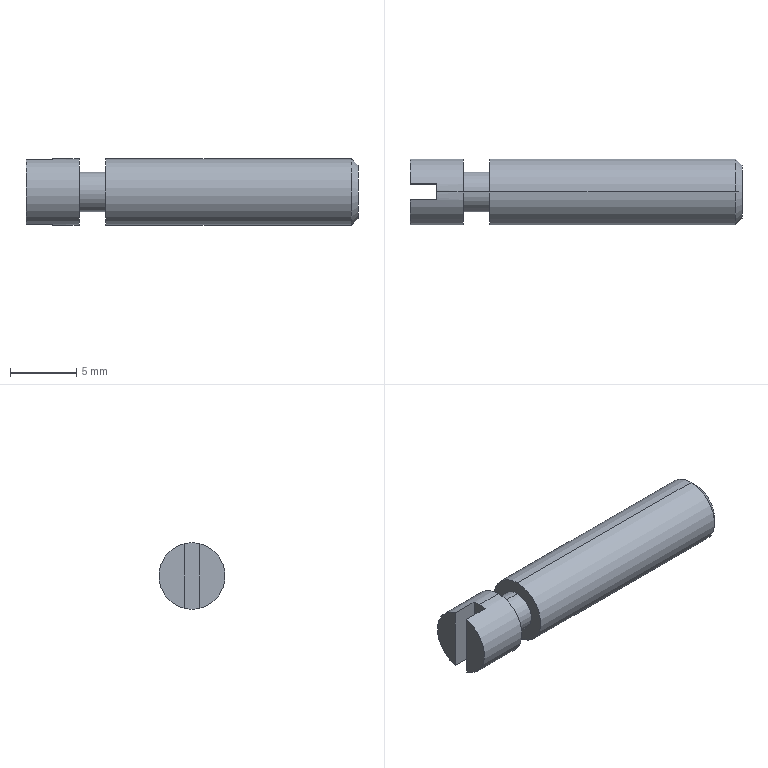Part | STEP file | QA-BSPO5_25b | 1 solid | 16 faces | box 25 x 5 x 5 mm | volume 452.091 mm3 | plane 8 | cylinder 6 | cone 2 | commonest cylinder face diameters 5 x4 3 x2
STEP:
#1=CARTESIAN_POINT('',(0.,0.,0.));
#2=DIRECTION('',(0.,0.,1.));
#3=DIRECTION('',(1.,0.,0.));
#4=AXIS2_PLACEMENT_3D('',#1,#2,#3);
#5=CARTESIAN_POINT('',(4.,0.,-2.5));
#6=VERTEX_POINT('',#5);
#7=CARTESIAN_POINT('',(4.,0.,2.5));
#8=VERTEX_POINT('',#7);
#9=CARTESIAN_POINT('',(4.,0.,0.));
#10=DIRECTION('',(1.,0.,0.));
#11=DIRECTION('',(0.,0.,-1.));
#12=AXIS2_PLACEMENT_3D('',#9,#10,#11);
#13=CIRCLE('',#12,2.5);
#14=CARTESIAN_POINT('',(25.,0.,0.));
#15=DIRECTION('',(-1.,0.,0.));
#16=DIRECTION('',(0.,0.,1.));
#17=AXIS2_PLACEMENT_3D('',#14,#15,#16);
#18=CYLINDRICAL_SURFACE('',#17,2.5);
#19=CARTESIAN_POINT('',(3.142,21.));
#20=DIRECTION('',(-1.,0.));
#21=VECTOR('',#20,1.);
#22=LINE('',#19,#21);
#23=(GEOMETRIC_REPRESENTATION_CONTEXT(2)PARAMETRIC_REPRESENTATION_CONTEXT()REPRESENTATION_CONTEXT('',''));
#24=DEFINITIONAL_REPRESENTATION('',(#22),#23);
#25=PCURVE('',#18,#24);
#26=CARTESIAN_POINT('',(4.,3.5,0.));
#27=DIRECTION('',(1.,0.,0.));
#28=DIRECTION('',(0.,0.,-1.));
#29=AXIS2_PLACEMENT_3D('',#26,#27,#28);
#30=PLANE('',#29);
#31=CARTESIAN_POINT('',(0.,-3.5));
#32=DIRECTION('',(1.,0.));
#33=AXIS2_PLACEMENT_2D('',#31,#32);
#34=CIRCLE('',#33,2.5);
#35=(GEOMETRIC_REPRESENTATION_CONTEXT(2)PARAMETRIC_REPRESENTATION_CONTEXT()REPRESENTATION_CONTEXT('',''));
#36=DEFINITIONAL_REPRESENTATION('',(#34),#35);
#37=PCURVE('',#30,#36);
#38=SURFACE_CURVE('',#13,(#25,#37),.PCURVE_S1.);
#39=EDGE_CURVE('',#6,#8,#38,.T.);
#40=ORIENTED_EDGE('',*,*,#39,.F.);
#41=CARTESIAN_POINT('',(2.,0.,-2.5));
#42=VERTEX_POINT('',#41);
#43=CARTESIAN_POINT('',(25.,0.,-2.5));
#44=DIRECTION('',(-1.,0.,0.));
#45=VECTOR('',#44,1.);
#46=LINE('',#43,#45);
#47=CARTESIAN_POINT('',(3.142,0.));
#48=DIRECTION('',(0.,1.));
#49=VECTOR('',#48,1.);
#50=LINE('',#47,#49);
#51=(GEOMETRIC_REPRESENTATION_CONTEXT(2)PARAMETRIC_REPRESENTATION_CONTEXT()REPRESENTATION_CONTEXT('',''));
#52=DEFINITIONAL_REPRESENTATION('',(#50),#51);
#53=PCURVE('',#18,#52);
#54=CARTESIAN_POINT('',(25.,0.,0.));
#55=DIRECTION('',(-1.,0.,0.));
#56=DIRECTION('',(0.,0.,1.));
#57=AXIS2_PLACEMENT_3D('',#54,#55,#56);
#58=CYLINDRICAL_SURFACE('',#57,2.5);
#59=CARTESIAN_POINT('',(3.142,0.));
#60=DIRECTION('',(0.,1.));
#61=VECTOR('',#60,1.);
#62=LINE('',#59,#61);
#63=(GEOMETRIC_REPRESENTATION_CONTEXT(2)PARAMETRIC_REPRESENTATION_CONTEXT()REPRESENTATION_CONTEXT('',''));
#64=DEFINITIONAL_REPRESENTATION('',(#62),#63);
#65=PCURVE('',#58,#64);
#66=SURFACE_CURVE('',#46,(#53,#65),.PCURVE_S1.);
#67=EDGE_CURVE('',#6,#42,#66,.T.);
#68=ORIENTED_EDGE('',*,*,#67,.T.);
#69=CARTESIAN_POINT('',(2.,0.6,-2.427));
#70=VERTEX_POINT('',#69);
#71=CARTESIAN_POINT('',(2.,0.,0.));
#72=DIRECTION('',(1.,0.,0.));
#73=DIRECTION('',(0.,0.,-1.));
#74=AXIS2_PLACEMENT_3D('',#71,#72,#73);
#75=CIRCLE('',#74,2.5);
#76=CARTESIAN_POINT('',(3.142,23.));
#77=DIRECTION('',(-1.,0.));
#78=VECTOR('',#77,1.);
#79=LINE('',#76,#78);
#80=(GEOMETRIC_REPRESENTATION_CONTEXT(2)PARAMETRIC_REPRESENTATION_CONTEXT()REPRESENTATION_CONTEXT('',''));
#81=DEFINITIONAL_REPRESENTATION('',(#79),#80);
#82=PCURVE('',#18,#81);
#83=CARTESIAN_POINT('',(2.,-0.6,-2.5));
#84=DIRECTION('',(1.,0.,0.));
#85=DIRECTION('',(0.,0.,-1.));
#86=AXIS2_PLACEMENT_3D('',#83,#84,#85);
#87=PLANE('',#86);
#88=CARTESIAN_POINT('',(-2.5,0.6));
#89=DIRECTION('',(1.,0.));
#90=AXIS2_PLACEMENT_2D('',#88,#89);
#91=CIRCLE('',#90,2.5);
#92=(GEOMETRIC_REPRESENTATION_CONTEXT(2)PARAMETRIC_REPRESENTATION_CONTEXT()REPRESENTATION_CONTEXT('',''));
#93=DEFINITIONAL_REPRESENTATION('',(#91),#92);
#94=PCURVE('',#87,#93);
#95=SURFACE_CURVE('',#75,(#82,#94),.PCURVE_S1.);
#96=EDGE_CURVE('',#42,#70,#95,.T.);
#97=ORIENTED_EDGE('',*,*,#96,.T.);
#98=CARTESIAN_POINT('',(0.,0.6,-2.427));
#99=VERTEX_POINT('',#98);
#100=CARTESIAN_POINT('',(25.,0.6,-2.427));
#101=DIRECTION('',(-1.,0.,0.));
#102=VECTOR('',#101,1.);
#103=LINE('',#100,#102);
#104=CARTESIAN_POINT('',(2.899,0.));
#105=DIRECTION('',(0.,1.));
#106=VECTOR('',#105,1.);
#107=LINE('',#104,#106);
#108=(GEOMETRIC_REPRESENTATION_CONTEXT(2)PARAMETRIC_REPRESENTATION_CONTEXT()REPRESENTATION_CONTEXT('',''));
#109=DEFINITIONAL_REPRESENTATION('',(#107),#108);
#110=PCURVE('',#18,#109);
#111=CARTESIAN_POINT('',(2.,0.6,-2.5));
#112=DIRECTION('',(0.,1.,0.));
#113=DIRECTION('',(0.,0.,1.));
#114=AXIS2_PLACEMENT_3D('',#111,#112,#113);
#115=PLANE('',#114);
#116=CARTESIAN_POINT('',(0.07307,23.));
#117=DIRECTION('',(0.,-1.));
#118=VECTOR('',#117,1.);
#119=LINE('',#116,#118);
#120=(GEOMETRIC_REPRESENTATION_CONTEXT(2)PARAMETRIC_REPRESENTATION_CONTEXT()REPRESENTATION_CONTEXT('',''));
#121=DEFINITIONAL_REPRESENTATION('',(#119),#120);
#122=PCURVE('',#115,#121);
#123=SURFACE_CURVE('',#103,(#110,#122),.PCURVE_S1.);
#124=EDGE_CURVE('',#70,#99,#123,.T.);
#125=ORIENTED_EDGE('',*,*,#124,.T.);
#126=CARTESIAN_POINT('',(0.,0.6,2.427));
#127=VERTEX_POINT('',#126);
#128=CARTESIAN_POINT('',(0.,0.,0.));
#129=DIRECTION('',(-1.,0.,0.));
#130=DIRECTION('',(0.,0.,1.));
#131=AXIS2_PLACEMENT_3D('',#128,#129,#130);
#132=CIRCLE('',#131,2.5);
#133=CARTESIAN_POINT('',(0.,25.));
#134=DIRECTION('',(1.,0.));
#135=VECTOR('',#134,1.);
#136=LINE('',#133,#135);
#137=(GEOMETRIC_REPRESENTATION_CONTEXT(2)PARAMETRIC_REPRESENTATION_CONTEXT()REPRESENTATION_CONTEXT('',''));
#138=DEFINITIONAL_REPRESENTATION('',(#136),#137);
#139=PCURVE('',#18,#138);
#140=CARTESIAN_POINT('',(0.,0.,0.));
#141=DIRECTION('',(1.,0.,0.));
#142=DIRECTION('',(0.,0.,-1.));
#143=AXIS2_PLACEMENT_3D('',#140,#141,#142);
#144=PLANE('',#143);
#145=CARTESIAN_POINT('',(-2.5,0.));
#146=CARTESIAN_POINT('',(-2.5,4.33));
#147=CARTESIAN_POINT('',(1.25,2.165));
#148=CARTESIAN_POINT('',(5.,0.));
#149=CARTESIAN_POINT('',(1.25,-2.165));
#150=CARTESIAN_POINT('',(-2.5,-4.33));
#151=CARTESIAN_POINT('',(-2.5,0.));
#152=(BOUNDED_CURVE()B_SPLINE_CURVE(2,(#145,#146,#147,#148,#149,#150,#151),.UNSPECIFIED.,.T.,.F.)B_SPLINE_CURVE_WITH_KNOTS((1,2,2,2,2,1),(-2.094,0.,2.094,4.189,6.283,8.378),.UNSPECIFIED.)CURVE()GEOMETRIC_REPRESENTATION_ITEM()RATIONAL_B_SPLINE_CURVE((1.,0.5,1.,0.5,1.,0.5,1.))REPRESENTATION_ITEM(''));
#153=(GEOMETRIC_REPRESENTATION_CONTEXT(2)PARAMETRIC_REPRESENTATION_CONTEXT()REPRESENTATION_CONTEXT('',''));
#154=DEFINITIONAL_REPRESENTATION('',(#152),#153);
#155=PCURVE('',#144,#154);
#156=SURFACE_CURVE('',#132,(#139,#155),.PCURVE_S1.);
#157=EDGE_CURVE('',#127,#99,#156,.T.);
#158=ORIENTED_EDGE('',*,*,#157,.F.);
#159=CARTESIAN_POINT('',(2.,0.6,2.427));
#160=VERTEX_POINT('',#159);
#161=CARTESIAN_POINT('',(25.,0.6,2.427));
#162=DIRECTION('',(1.,0.,0.));
#163=VECTOR('',#162,1.);
#164=LINE('',#161,#163);
#165=CARTESIAN_POINT('',(0.2424,0.));
#166=DIRECTION('',(0.,-1.));
#167=VECTOR('',#166,1.);
#168=LINE('',#165,#167);
#169=(GEOMETRIC_REPRESENTATION_CONTEXT(2)PARAMETRIC_REPRESENTATION_CONTEXT()REPRESENTATION_CONTEXT('',''));
#170=DEFINITIONAL_REPRESENTATION('',(#168),#169);
#171=PCURVE('',#18,#170);
#172=CARTESIAN_POINT('',(4.927,23.));
#173=DIRECTION('',(0.,1.));
#174=VECTOR('',#173,1.);
#175=LINE('',#172,#174);
#176=(GEOMETRIC_REPRESENTATION_CONTEXT(2)PARAMETRIC_REPRESENTATION_CONTEXT()REPRESENTATION_CONTEXT('',''));
#177=DEFINITIONAL_REPRESENTATION('',(#175),#176);
#178=PCURVE('',#115,#177);
#179=SURFACE_CURVE('',#164,(#171,#178),.PCURVE_S1.);
#180=EDGE_CURVE('',#127,#160,#179,.T.);
#181=ORIENTED_EDGE('',*,*,#180,.T.);
#182=CARTESIAN_POINT('',(2.,0.,2.5));
#183=VERTEX_POINT('',#182);
#184=CARTESIAN_POINT('',(2.,0.,0.));
#185=DIRECTION('',(1.,0.,0.));
#186=DIRECTION('',(0.,0.,-1.));
#187=AXIS2_PLACEMENT_3D('',#184,#185,#186);
#188=CIRCLE('',#187,2.5);
#189=CARTESIAN_POINT('',(3.142,23.));
#190=DIRECTION('',(-1.,0.));
#191=VECTOR('',#190,1.);
#192=LINE('',#189,#191);
#193=(GEOMETRIC_REPRESENTATION_CONTEXT(2)PARAMETRIC_REPRESENTATION_CONTEXT()REPRESENTATION_CONTEXT('',''));
#194=DEFINITIONAL_REPRESENTATION('',(#192),#193);
#195=PCURVE('',#18,#194);
#196=CARTESIAN_POINT('',(-2.5,0.6));
#197=DIRECTION('',(1.,0.));
#198=AXIS2_PLACEMENT_2D('',#196,#197);
#199=CIRCLE('',#198,2.5);
#200=(GEOMETRIC_REPRESENTATION_CONTEXT(2)PARAMETRIC_REPRESENTATION_CONTEXT()REPRESENTATION_CONTEXT('',''));
#201=DEFINITIONAL_REPRESENTATION('',(#199),#200);
#202=PCURVE('',#87,#201);
#203=SURFACE_CURVE('',#188,(#195,#202),.PCURVE_S1.);
#204=EDGE_CURVE('',#160,#183,#203,.T.);
#205=ORIENTED_EDGE('',*,*,#204,.T.);
#206=CARTESIAN_POINT('',(25.,0.,2.5));
#207=DIRECTION('',(-1.,0.,0.));
#208=VECTOR('',#207,1.);
#209=LINE('',#206,#208);
#210=CARTESIAN_POINT('',(0.,0.));
#211=DIRECTION('',(0.,1.));
#212=VECTOR('',#211,1.);
#213=LINE('',#210,#212);
#214=(GEOMETRIC_REPRESENTATION_CONTEXT(2)PARAMETRIC_REPRESENTATION_CONTEXT()REPRESENTATION_CONTEXT('',''));
#215=DEFINITIONAL_REPRESENTATION('',(#213),#214);
#216=PCURVE('',#18,#215);
#217=CARTESIAN_POINT('',(6.283,0.));
#218=DIRECTION('',(0.,1.));
#219=VECTOR('',#218,1.);
#220=LINE('',#217,#219);
#221=(GEOMETRIC_REPRESENTATION_CONTEXT(2)PARAMETRIC_REPRESENTATION_CONTEXT()REPRESENTATION_CONTEXT('',''));
#222=DEFINITIONAL_REPRESENTATION('',(#220),#221);
#223=PCURVE('',#58,#222);
#224=SURFACE_CURVE('',#209,(#216,#223),.PCURVE_S1.);
#225=EDGE_CURVE('',#8,#183,#224,.T.);
#226=ORIENTED_EDGE('',*,*,#225,.F.);
#227=EDGE_LOOP('',(#40,#68,#97,#125,#158,#181,#205,#226));
#228=FACE_BOUND('',#227,.T.);
#229=ADVANCED_FACE('',(#228),#18,.T.);
#230=CARTESIAN_POINT('',(6.,0.,1.5));
#231=VERTEX_POINT('',#230);
#232=CARTESIAN_POINT('',(6.,0.,-1.5));
#233=VERTEX_POINT('',#232);
#234=CARTESIAN_POINT('',(6.,0.,0.));
#235=DIRECTION('',(-1.,0.,0.));
#236=DIRECTION('',(0.,0.,1.));
#237=AXIS2_PLACEMENT_3D('',#234,#235,#236);
#238=CIRCLE('',#237,1.5);
#239=CARTESIAN_POINT('',(5.,0.,0.));
#240=DIRECTION('',(-1.,0.,0.));
#241=DIRECTION('',(0.,0.,1.));
#242=AXIS2_PLACEMENT_3D('',#239,#240,#241);
#243=CYLINDRICAL_SURFACE('',#242,1.5);
#244=CARTESIAN_POINT('',(0.,-1.));
#245=DIRECTION('',(1.,0.));
#246=VECTOR('',#245,1.);
#247=LINE('',#244,#246);
#248=(GEOMETRIC_REPRESENTATION_CONTEXT(2)PARAMETRIC_REPRESENTATION_CONTEXT()REPRESENTATION_CONTEXT('',''));
#249=DEFINITIONAL_REPRESENTATION('',(#247),#248);
#250=PCURVE('',#243,#249);
#251=CARTESIAN_POINT('',(6.,1.5,0.));
#252=DIRECTION('',(-1.,0.,0.));
#253=DIRECTION('',(0.,0.,1.));
#254=AXIS2_PLACEMENT_3D('',#251,#252,#253);
#255=PLANE('',#254);
#256=CARTESIAN_POINT('',(0.,-1.5));
#257=DIRECTION('',(1.,0.));
#258=AXIS2_PLACEMENT_2D('',#256,#257);
#259=CIRCLE('',#258,1.5);
#260=(GEOMETRIC_REPRESENTATION_CONTEXT(2)PARAMETRIC_REPRESENTATION_CONTEXT()REPRESENTATION_CONTEXT('',''));
#261=DEFINITIONAL_REPRESENTATION('',(#259),#260);
#262=PCURVE('',#255,#261);
#263=SURFACE_CURVE('',#238,(#250,#262),.PCURVE_S1.);
#264=EDGE_CURVE('',#231,#233,#263,.T.);
#265=ORIENTED_EDGE('',*,*,#264,.T.);
#266=CARTESIAN_POINT('',(4.,0.,-1.5));
#267=VERTEX_POINT('',#266);
#268=CARTESIAN_POINT('',(5.,0.,-1.5));
#269=DIRECTION('',(-1.,0.,0.));
#270=VECTOR('',#269,1.);
#271=LINE('',#268,#270);
#272=CARTESIAN_POINT('',(3.142,0.));
#273=DIRECTION('',(0.,1.));
#274=VECTOR('',#273,1.);
#275=LINE('',#272,#274);
#276=(GEOMETRIC_REPRESENTATION_CONTEXT(2)PARAMETRIC_REPRESENTATION_CONTEXT()REPRESENTATION_CONTEXT('',''));
#277=DEFINITIONAL_REPRESENTATION('',(#275),#276);
#278=PCURVE('',#243,#277);
#279=CARTESIAN_POINT('',(5.,0.,0.));
#280=DIRECTION('',(-1.,0.,0.));
#281=DIRECTION('',(0.,0.,1.));
#282=AXIS2_PLACEMENT_3D('',#279,#280,#281);
#283=CYLINDRICAL_SURFACE('',#282,1.5);
#284=CARTESIAN_POINT('',(3.142,0.));
#285=DIRECTION('',(0.,1.));
#286=VECTOR('',#285,1.);
#287=LINE('',#284,#286);
#288=(GEOMETRIC_REPRESENTATION_CONTEXT(2)PARAMETRIC_REPRESENTATION_CONTEXT()REPRESENTATION_CONTEXT('',''));
#289=DEFINITIONAL_REPRESENTATION('',(#287),#288);
#290=PCURVE('',#283,#289);
#291=SURFACE_CURVE('',#271,(#278,#290),.PCURVE_S1.);
#292=EDGE_CURVE('',#233,#267,#291,.T.);
#293=ORIENTED_EDGE('',*,*,#292,.T.);
#294=CARTESIAN_POINT('',(4.,0.,1.5));
#295=VERTEX_POINT('',#294);
#296=CARTESIAN_POINT('',(4.,0.,0.));
#297=DIRECTION('',(-1.,0.,0.));
#298=DIRECTION('',(0.,0.,1.));
#299=AXIS2_PLACEMENT_3D('',#296,#297,#298);
#300=CIRCLE('',#299,1.5);
#301=CARTESIAN_POINT('',(0.,1.));
#302=DIRECTION('',(1.,0.));
#303=VECTOR('',#302,1.);
#304=LINE('',#301,#303);
#305=(GEOMETRIC_REPRESENTATION_CONTEXT(2)PARAMETRIC_REPRESENTATION_CONTEXT()REPRESENTATION_CONTEXT('',''));
#306=DEFINITIONAL_REPRESENTATION('',(#304),#305);
#307=PCURVE('',#243,#306);
#308=CARTESIAN_POINT('',(-1.5,-3.5));
#309=CARTESIAN_POINT('',(-1.5,-0.9019));
#310=CARTESIAN_POINT('',(0.75,-2.201));
#311=CARTESIAN_POINT('',(3.,-3.5));
#312=CARTESIAN_POINT('',(0.75,-4.799));
#313=CARTESIAN_POINT('',(-1.5,-6.098));
#314=CARTESIAN_POINT('',(-1.5,-3.5));
#315=(BOUNDED_CURVE()B_SPLINE_CURVE(2,(#308,#309,#310,#311,#312,#313,#314),.UNSPECIFIED.,.T.,.F.)B_SPLINE_CURVE_WITH_KNOTS((1,2,2,2,2,1),(-2.094,0.,2.094,4.189,6.283,8.378),.UNSPECIFIED.)CURVE()GEOMETRIC_REPRESENTATION_ITEM()RATIONAL_B_SPLINE_CURVE((1.,0.5,1.,0.5,1.,0.5,1.))REPRESENTATION_ITEM(''));
#316=(GEOMETRIC_REPRESENTATION_CONTEXT(2)PARAMETRIC_REPRESENTATION_CONTEXT()REPRESENTATION_CONTEXT('',''));
#317=DEFINITIONAL_REPRESENTATION('',(#315),#316);
#318=PCURVE('',#30,#317);
#319=SURFACE_CURVE('',#300,(#307,#318),.PCURVE_S1.);
#320=EDGE_CURVE('',#295,#267,#319,.T.);
#321=ORIENTED_EDGE('',*,*,#320,.F.);
#322=CARTESIAN_POINT('',(5.,0.,1.5));
#323=DIRECTION('',(-1.,0.,0.));
#324=VECTOR('',#323,1.);
#325=LINE('',#322,#324);
#326=CARTESIAN_POINT('',(0.,0.));
#327=DIRECTION('',(0.,1.));
#328=VECTOR('',#327,1.);
#329=LINE('',#326,#328);
#330=(GEOMETRIC_REPRESENTATION_CONTEXT(2)PARAMETRIC_REPRESENTATION_CONTEXT()REPRESENTATION_CONTEXT('',''));
#331=DEFINITIONAL_REPRESENTATION('',(#329),#330);
#332=PCURVE('',#243,#331);
#333=CARTESIAN_POINT('',(6.283,0.));
#334=DIRECTION('',(0.,1.));
#335=VECTOR('',#334,1.);
#336=LINE('',#333,#335);
#337=(GEOMETRIC_REPRESENTATION_CONTEXT(2)PARAMETRIC_REPRESENTATION_CONTEXT()REPRESENTATION_CONTEXT('',''));
#338=DEFINITIONAL_REPRESENTATION('',(#336),#337);
#339=PCURVE('',#283,#338);
#340=SURFACE_CURVE('',#325,(#332,#339),.PCURVE_S1.);
#341=EDGE_CURVE('',#231,#295,#340,.T.);
#342=ORIENTED_EDGE('',*,*,#341,.F.);
#343=EDGE_LOOP('',(#265,#293,#321,#342));
#344=FACE_BOUND('',#343,.T.);
#345=ADVANCED_FACE('',(#344),#243,.T.);
#346=CARTESIAN_POINT('',(25.,0.,2.01));
#347=VERTEX_POINT('',#346);
#348=CARTESIAN_POINT('',(25.,0.,-2.01));
#349=VERTEX_POINT('',#348);
#350=CARTESIAN_POINT('',(25.,0.,0.));
#351=DIRECTION('',(-1.,0.,0.));
#352=DIRECTION('',(0.,0.,1.));
#353=AXIS2_PLACEMENT_3D('',#350,#351,#352);
#354=CIRCLE('',#353,2.01);
#355=CARTESIAN_POINT('',(25.,0.,0.));
#356=DIRECTION('',(-1.,0.,0.));
#357=DIRECTION('',(0.,0.,1.));
#358=AXIS2_PLACEMENT_3D('',#355,#356,#357);
#359=CONICAL_SURFACE('',#358,2.01,0.7854);
#360=CARTESIAN_POINT('',(0.,0.));
#361=DIRECTION('',(1.,0.));
#362=VECTOR('',#361,1.);
#363=LINE('',#360,#362);
#364=(GEOMETRIC_REPRESENTATION_CONTEXT(2)PARAMETRIC_REPRESENTATION_CONTEXT()REPRESENTATION_CONTEXT('',''));
#365=DEFINITIONAL_REPRESENTATION('',(#363),#364);
#366=PCURVE('',#359,#365);
#367=CARTESIAN_POINT('',(25.,2.01,0.));
#368=DIRECTION('',(-1.,0.,0.));
#369=DIRECTION('',(0.,0.,1.));
#370=AXIS2_PLACEMENT_3D('',#367,#368,#369);
#371=PLANE('',#370);
#372=CARTESIAN_POINT('',(0.,-2.01));
#373=DIRECTION('',(1.,0.));
#374=AXIS2_PLACEMENT_2D('',#372,#373);
#375=CIRCLE('',#374,2.01);
#376=(GEOMETRIC_REPRESENTATION_CONTEXT(2)PARAMETRIC_REPRESENTATION_CONTEXT()REPRESENTATION_CONTEXT('',''));
#377=DEFINITIONAL_REPRESENTATION('',(#375),#376);
#378=PCURVE('',#371,#377);
#379=SURFACE_CURVE('',#354,(#366,#378),.PCURVE_S1.);
#380=EDGE_CURVE('',#347,#349,#379,.T.);
#381=ORIENTED_EDGE('',*,*,#380,.T.);
#382=CARTESIAN_POINT('',(24.509,0.,-2.5));
#383=VERTEX_POINT('',#382);
#384=CARTESIAN_POINT('',(25.,0.,-2.01));
#385=DIRECTION('',(-0.7071,0.,-0.7071));
#386=VECTOR('',#385,1.);
#387=LINE('',#384,#386);
#388=CARTESIAN_POINT('',(3.142,0.));
#389=DIRECTION('',(0.,1.));
#390=VECTOR('',#389,1.);
#391=LINE('',#388,#390);
#392=(GEOMETRIC_REPRESENTATION_CONTEXT(2)PARAMETRIC_REPRESENTATION_CONTEXT()REPRESENTATION_CONTEXT('',''));
#393=DEFINITIONAL_REPRESENTATION('',(#391),#392);
#394=PCURVE('',#359,#393);
#395=CARTESIAN_POINT('',(25.,0.,0.));
#396=DIRECTION('',(-1.,0.,0.));
#397=DIRECTION('',(0.,0.,1.));
#398=AXIS2_PLACEMENT_3D('',#395,#396,#397);
#399=CONICAL_SURFACE('',#398,2.01,0.7854);
#400=CARTESIAN_POINT('',(3.142,0.));
#401=DIRECTION('',(0.,1.));
#402=VECTOR('',#401,1.);
#403=LINE('',#400,#402);
#404=(GEOMETRIC_REPRESENTATION_CONTEXT(2)PARAMETRIC_REPRESENTATION_CONTEXT()REPRESENTATION_CONTEXT('',''));
#405=DEFINITIONAL_REPRESENTATION('',(#403),#404);
#406=PCURVE('',#399,#405);
#407=SURFACE_CURVE('',#387,(#394,#406),.PCURVE_S1.);
#408=EDGE_CURVE('',#349,#383,#407,.T.);
#409=ORIENTED_EDGE('',*,*,#408,.T.);
#410=CARTESIAN_POINT('',(24.509,0.,2.5));
#411=VERTEX_POINT('',#410);
#412=CARTESIAN_POINT('',(24.509,0.,0.));
#413=DIRECTION('',(-1.,0.,0.));
#414=DIRECTION('',(0.,0.,1.));
#415=AXIS2_PLACEMENT_3D('',#412,#413,#414);
#416=CIRCLE('',#415,2.5);
#417=CARTESIAN_POINT('',(0.,0.4905));
#418=DIRECTION('',(1.,0.));
#419=VECTOR('',#418,1.);
#420=LINE('',#417,#419);
#421=(GEOMETRIC_REPRESENTATION_CONTEXT(2)PARAMETRIC_REPRESENTATION_CONTEXT()REPRESENTATION_CONTEXT('',''));
#422=DEFINITIONAL_REPRESENTATION('',(#420),#421);
#423=PCURVE('',#359,#422);
#424=CARTESIAN_POINT('',(25.,0.,0.));
#425=DIRECTION('',(-1.,0.,0.));
#426=DIRECTION('',(0.,0.,1.));
#427=AXIS2_PLACEMENT_3D('',#424,#425,#426);
#428=CYLINDRICAL_SURFACE('',#427,2.5);
#429=CARTESIAN_POINT('',(0.,0.4905));
#430=DIRECTION('',(1.,0.));
#431=VECTOR('',#430,1.);
#432=LINE('',#429,#431);
#433=(GEOMETRIC_REPRESENTATION_CONTEXT(2)PARAMETRIC_REPRESENTATION_CONTEXT()REPRESENTATION_CONTEXT('',''));
#434=DEFINITIONAL_REPRESENTATION('',(#432),#433);
#435=PCURVE('',#428,#434);
#436=SURFACE_CURVE('',#416,(#423,#435),.PCURVE_S1.);
#437=EDGE_CURVE('',#411,#383,#436,.T.);
#438=ORIENTED_EDGE('',*,*,#437,.F.);
#439=CARTESIAN_POINT('',(25.,0.,2.01));
#440=DIRECTION('',(-0.7071,0.,0.7071));
#441=VECTOR('',#440,1.);
#442=LINE('',#439,#441);
#443=CARTESIAN_POINT('',(0.,0.));
#444=DIRECTION('',(0.,1.));
#445=VECTOR('',#444,1.);
#446=LINE('',#443,#445);
#447=(GEOMETRIC_REPRESENTATION_CONTEXT(2)PARAMETRIC_REPRESENTATION_CONTEXT()REPRESENTATION_CONTEXT('',''));
#448=DEFINITIONAL_REPRESENTATION('',(#446),#447);
#449=PCURVE('',#359,#448);
#450=CARTESIAN_POINT('',(6.283,0.));
#451=DIRECTION('',(0.,1.));
#452=VECTOR('',#451,1.);
#453=LINE('',#450,#452);
#454=(GEOMETRIC_REPRESENTATION_CONTEXT(2)PARAMETRIC_REPRESENTATION_CONTEXT()REPRESENTATION_CONTEXT('',''));
#455=DEFINITIONAL_REPRESENTATION('',(#453),#454);
#456=PCURVE('',#399,#455);
#457=SURFACE_CURVE('',#442,(#449,#456),.PCURVE_S1.);
#458=EDGE_CURVE('',#347,#411,#457,.T.);
#459=ORIENTED_EDGE('',*,*,#458,.F.);
#460=EDGE_LOOP('',(#381,#409,#438,#459));
#461=FACE_BOUND('',#460,.T.);
#462=ADVANCED_FACE('',(#461),#359,.T.);
#463=ORIENTED_EDGE('',*,*,#437,.T.);
#464=CARTESIAN_POINT('',(6.,0.,-2.5));
#465=VERTEX_POINT('',#464);
#466=CARTESIAN_POINT('',(25.,0.,-2.5));
#467=DIRECTION('',(-1.,0.,0.));
#468=VECTOR('',#467,1.);
#469=LINE('',#466,#468);
#470=CARTESIAN_POINT('',(3.142,0.));
#471=DIRECTION('',(0.,1.));
#472=VECTOR('',#471,1.);
#473=LINE('',#470,#472);
#474=(GEOMETRIC_REPRESENTATION_CONTEXT(2)PARAMETRIC_REPRESENTATION_CONTEXT()REPRESENTATION_CONTEXT('',''));
#475=DEFINITIONAL_REPRESENTATION('',(#473),#474);
#476=PCURVE('',#428,#475);
#477=CARTESIAN_POINT('',(25.,0.,0.));
#478=DIRECTION('',(-1.,0.,0.));
#479=DIRECTION('',(0.,0.,1.));
#480=AXIS2_PLACEMENT_3D('',#477,#478,#479);
#481=CYLINDRICAL_SURFACE('',#480,2.5);
#482=CARTESIAN_POINT('',(3.142,0.));
#483=DIRECTION('',(0.,1.));
#484=VECTOR('',#483,1.);
#485=LINE('',#482,#484);
#486=(GEOMETRIC_REPRESENTATION_CONTEXT(2)PARAMETRIC_REPRESENTATION_CONTEXT()REPRESENTATION_CONTEXT('',''));
#487=DEFINITIONAL_REPRESENTATION('',(#485),#486);
#488=PCURVE('',#481,#487);
#489=SURFACE_CURVE('',#469,(#476,#488),.PCURVE_S1.);
#490=EDGE_CURVE('',#383,#465,#489,.T.);
#491=ORIENTED_EDGE('',*,*,#490,.T.);
#492=CARTESIAN_POINT('',(6.,0.,2.5));
#493=VERTEX_POINT('',#492);
#494=CARTESIAN_POINT('',(6.,0.,0.));
#495=DIRECTION('',(-1.,0.,0.));
#496=DIRECTION('',(0.,0.,1.));
#497=AXIS2_PLACEMENT_3D('',#494,#495,#496);
#498=CIRCLE('',#497,2.5);
#499=CARTESIAN_POINT('',(0.,19.));
#500=DIRECTION('',(1.,0.));
#501=VECTOR('',#500,1.);
#502=LINE('',#499,#501);
#503=(GEOMETRIC_REPRESENTATION_CONTEXT(2)PARAMETRIC_REPRESENTATION_CONTEXT()REPRESENTATION_CONTEXT('',''));
#504=DEFINITIONAL_REPRESENTATION('',(#502),#503);
#505=PCURVE('',#428,#504);
#506=CARTESIAN_POINT('',(0.,-1.5));
#507=DIRECTION('',(1.,0.));
#508=AXIS2_PLACEMENT_2D('',#506,#507);
#509=CIRCLE('',#508,2.5);
#510=(GEOMETRIC_REPRESENTATION_CONTEXT(2)PARAMETRIC_REPRESENTATION_CONTEXT()REPRESENTATION_CONTEXT('',''));
#511=DEFINITIONAL_REPRESENTATION('',(#509),#510);
#512=PCURVE('',#255,#511);
#513=SURFACE_CURVE('',#498,(#505,#512),.PCURVE_S1.);
#514=EDGE_CURVE('',#493,#465,#513,.T.);
#515=ORIENTED_EDGE('',*,*,#514,.F.);
#516=CARTESIAN_POINT('',(25.,0.,2.5));
#517=DIRECTION('',(-1.,0.,0.));
#518=VECTOR('',#517,1.);
#519=LINE('',#516,#518);
#520=CARTESIAN_POINT('',(0.,0.));
#521=DIRECTION('',(0.,1.));
#522=VECTOR('',#521,1.);
#523=LINE('',#520,#522);
#524=(GEOMETRIC_REPRESENTATION_CONTEXT(2)PARAMETRIC_REPRESENTATION_CONTEXT()REPRESENTATION_CONTEXT('',''));
#525=DEFINITIONAL_REPRESENTATION('',(#523),#524);
#526=PCURVE('',#428,#525);
#527=CARTESIAN_POINT('',(6.283,0.));
#528=DIRECTION('',(0.,1.));
#529=VECTOR('',#528,1.);
#530=LINE('',#527,#529);
#531=(GEOMETRIC_REPRESENTATION_CONTEXT(2)PARAMETRIC_REPRESENTATION_CONTEXT()REPRESENTATION_CONTEXT('',''));
#532=DEFINITIONAL_REPRESENTATION('',(#530),#531);
#533=PCURVE('',#481,#532);
#534=SURFACE_CURVE('',#519,(#526,#533),.PCURVE_S1.);
#535=EDGE_CURVE('',#411,#493,#534,.T.);
#536=ORIENTED_EDGE('',*,*,#535,.F.);
#537=EDGE_LOOP('',(#463,#491,#515,#536));
#538=FACE_BOUND('',#537,.T.);
#539=ADVANCED_FACE('',(#538),#428,.T.);
#540=ORIENTED_EDGE('',*,*,#490,.F.);
#541=CARTESIAN_POINT('',(24.509,0.,0.));
#542=DIRECTION('',(-1.,0.,0.));
#543=DIRECTION('',(0.,0.,1.));
#544=AXIS2_PLACEMENT_3D('',#541,#542,#543);
#545=CIRCLE('',#544,2.5);
#546=CARTESIAN_POINT('',(0.,0.4905));
#547=DIRECTION('',(1.,0.));
#548=VECTOR('',#547,1.);
#549=LINE('',#546,#548);
#550=(GEOMETRIC_REPRESENTATION_CONTEXT(2)PARAMETRIC_REPRESENTATION_CONTEXT()REPRESENTATION_CONTEXT('',''));
#551=DEFINITIONAL_REPRESENTATION('',(#549),#550);
#552=PCURVE('',#481,#551);
#553=CARTESIAN_POINT('',(0.,0.4905));
#554=DIRECTION('',(1.,0.));
#555=VECTOR('',#554,1.);
#556=LINE('',#553,#555);
#557=(GEOMETRIC_REPRESENTATION_CONTEXT(2)PARAMETRIC_REPRESENTATION_CONTEXT()REPRESENTATION_CONTEXT('',''));
#558=DEFINITIONAL_REPRESENTATION('',(#556),#557);
#559=PCURVE('',#399,#558);
#560=SURFACE_CURVE('',#545,(#552,#559),.PCURVE_S1.);
#561=EDGE_CURVE('',#383,#411,#560,.T.);
#562=ORIENTED_EDGE('',*,*,#561,.T.);
#563=ORIENTED_EDGE('',*,*,#535,.T.);
#564=CARTESIAN_POINT('',(6.,0.,0.));
#565=DIRECTION('',(-1.,0.,0.));
#566=DIRECTION('',(0.,0.,1.));
#567=AXIS2_PLACEMENT_3D('',#564,#565,#566);
#568=CIRCLE('',#567,2.5);
#569=CARTESIAN_POINT('',(0.,19.));
#570=DIRECTION('',(1.,0.));
#571=VECTOR('',#570,1.);
#572=LINE('',#569,#571);
#573=(GEOMETRIC_REPRESENTATION_CONTEXT(2)PARAMETRIC_REPRESENTATION_CONTEXT()REPRESENTATION_CONTEXT('',''));
#574=DEFINITIONAL_REPRESENTATION('',(#572),#573);
#575=PCURVE('',#481,#574);
#576=CARTESIAN_POINT('',(0.,-1.5));
#577=DIRECTION('',(1.,0.));
#578=AXIS2_PLACEMENT_2D('',#576,#577);
#579=CIRCLE('',#578,2.5);
#580=(GEOMETRIC_REPRESENTATION_CONTEXT(2)PARAMETRIC_REPRESENTATION_CONTEXT()REPRESENTATION_CONTEXT('',''));
#581=DEFINITIONAL_REPRESENTATION('',(#579),#580);
#582=PCURVE('',#255,#581);
#583=SURFACE_CURVE('',#568,(#575,#582),.PCURVE_S1.);
#584=EDGE_CURVE('',#465,#493,#583,.T.);
#585=ORIENTED_EDGE('',*,*,#584,.F.);
#586=EDGE_LOOP('',(#540,#562,#563,#585));
#587=FACE_BOUND('',#586,.T.);
#588=ADVANCED_FACE('',(#587),#481,.T.);
#589=ORIENTED_EDGE('',*,*,#408,.F.);
#590=CARTESIAN_POINT('',(25.,0.,0.));
#591=DIRECTION('',(-1.,0.,0.));
#592=DIRECTION('',(0.,0.,1.));
#593=AXIS2_PLACEMENT_3D('',#590,#591,#592);
#594=CIRCLE('',#593,2.01);
#595=CARTESIAN_POINT('',(0.,0.));
#596=DIRECTION('',(1.,0.));
#597=VECTOR('',#596,1.);
#598=LINE('',#595,#597);
#599=(GEOMETRIC_REPRESENTATION_CONTEXT(2)PARAMETRIC_REPRESENTATION_CONTEXT()REPRESENTATION_CONTEXT('',''));
#600=DEFINITIONAL_REPRESENTATION('',(#598),#599);
#601=PCURVE('',#399,#600);
#602=CARTESIAN_POINT('',(0.,-2.01));
#603=DIRECTION('',(1.,0.));
#604=AXIS2_PLACEMENT_2D('',#602,#603);
#605=CIRCLE('',#604,2.01);
#606=(GEOMETRIC_REPRESENTATION_CONTEXT(2)PARAMETRIC_REPRESENTATION_CONTEXT()REPRESENTATION_CONTEXT('',''));
#607=DEFINITIONAL_REPRESENTATION('',(#605),#606);
#608=PCURVE('',#371,#607);
#609=SURFACE_CURVE('',#594,(#601,#608),.PCURVE_S1.);
#610=EDGE_CURVE('',#349,#347,#609,.T.);
#611=ORIENTED_EDGE('',*,*,#610,.T.);
#612=ORIENTED_EDGE('',*,*,#458,.T.);
#613=ORIENTED_EDGE('',*,*,#561,.F.);
#614=EDGE_LOOP('',(#589,#611,#612,#613));
#615=FACE_BOUND('',#614,.T.);
#616=ADVANCED_FACE('',(#615),#399,.T.);
#617=ORIENTED_EDGE('',*,*,#380,.F.);
#618=ORIENTED_EDGE('',*,*,#610,.F.);
#619=EDGE_LOOP('',(#617,#618));
#620=FACE_BOUND('',#619,.T.);
#621=ADVANCED_FACE('',(#620),#371,.F.);
#622=ORIENTED_EDGE('',*,*,#320,.T.);
#623=CARTESIAN_POINT('',(4.,0.,0.));
#624=DIRECTION('',(-1.,0.,0.));
#625=DIRECTION('',(0.,0.,1.));
#626=AXIS2_PLACEMENT_3D('',#623,#624,#625);
#627=CIRCLE('',#626,1.5);
#628=CARTESIAN_POINT('',(-1.5,-3.5));
#629=CARTESIAN_POINT('',(-1.5,-0.9019));
#630=CARTESIAN_POINT('',(0.75,-2.201));
#631=CARTESIAN_POINT('',(3.,-3.5));
#632=CARTESIAN_POINT('',(0.75,-4.799));
#633=CARTESIAN_POINT('',(-1.5,-6.098));
#634=CARTESIAN_POINT('',(-1.5,-3.5));
#635=(BOUNDED_CURVE()B_SPLINE_CURVE(2,(#628,#629,#630,#631,#632,#633,#634),.UNSPECIFIED.,.T.,.F.)B_SPLINE_CURVE_WITH_KNOTS((1,2,2,2,2,1),(-2.094,0.,2.094,4.189,6.283,8.378),.UNSPECIFIED.)CURVE()GEOMETRIC_REPRESENTATION_ITEM()RATIONAL_B_SPLINE_CURVE((1.,0.5,1.,0.5,1.,0.5,1.))REPRESENTATION_ITEM(''));
#636=(GEOMETRIC_REPRESENTATION_CONTEXT(2)PARAMETRIC_REPRESENTATION_CONTEXT()REPRESENTATION_CONTEXT('',''));
#637=DEFINITIONAL_REPRESENTATION('',(#635),#636);
#638=PCURVE('',#30,#637);
#639=CARTESIAN_POINT('',(0.,1.));
#640=DIRECTION('',(1.,0.));
#641=VECTOR('',#640,1.);
#642=LINE('',#639,#641);
#643=(GEOMETRIC_REPRESENTATION_CONTEXT(2)PARAMETRIC_REPRESENTATION_CONTEXT()REPRESENTATION_CONTEXT('',''));
#644=DEFINITIONAL_REPRESENTATION('',(#642),#643);
#645=PCURVE('',#283,#644);
#646=SURFACE_CURVE('',#627,(#638,#645),.PCURVE_S1.);
#647=EDGE_CURVE('',#267,#295,#646,.T.);
#648=ORIENTED_EDGE('',*,*,#647,.T.);
#649=EDGE_LOOP('',(#622,#648));
#650=FACE_BOUND('',#649,.T.);
#651=CARTESIAN_POINT('',(4.,0.,0.));
#652=DIRECTION('',(1.,0.,0.));
#653=DIRECTION('',(0.,0.,-1.));
#654=AXIS2_PLACEMENT_3D('',#651,#652,#653);
#655=CIRCLE('',#654,2.5);
#656=CARTESIAN_POINT('',(0.,-3.5));
#657=DIRECTION('',(1.,0.));
#658=AXIS2_PLACEMENT_2D('',#656,#657);
#659=CIRCLE('',#658,2.5);
#660=(GEOMETRIC_REPRESENTATION_CONTEXT(2)PARAMETRIC_REPRESENTATION_CONTEXT()REPRESENTATION_CONTEXT('',''));
#661=DEFINITIONAL_REPRESENTATION('',(#659),#660);
#662=PCURVE('',#30,#661);
#663=CARTESIAN_POINT('',(9.425,21.));
#664=DIRECTION('',(-1.,0.));
#665=VECTOR('',#664,1.);
#666=LINE('',#663,#665);
#667=(GEOMETRIC_REPRESENTATION_CONTEXT(2)PARAMETRIC_REPRESENTATION_CONTEXT()REPRESENTATION_CONTEXT('',''));
#668=DEFINITIONAL_REPRESENTATION('',(#666),#667);
#669=PCURVE('',#58,#668);
#670=SURFACE_CURVE('',#655,(#662,#669),.PCURVE_S1.);
#671=EDGE_CURVE('',#8,#6,#670,.T.);
#672=ORIENTED_EDGE('',*,*,#671,.T.);
#673=ORIENTED_EDGE('',*,*,#39,.T.);
#674=EDGE_LOOP('',(#672,#673));
#675=FACE_BOUND('',#674,.T.);
#676=ADVANCED_FACE('',(#650,#675),#30,.T.);
#677=ORIENTED_EDGE('',*,*,#264,.F.);
#678=CARTESIAN_POINT('',(6.,0.,0.));
#679=DIRECTION('',(-1.,0.,0.));
#680=DIRECTION('',(0.,0.,1.));
#681=AXIS2_PLACEMENT_3D('',#678,#679,#680);
#682=CIRCLE('',#681,1.5);
#683=CARTESIAN_POINT('',(0.,-1.5));
#684=DIRECTION('',(1.,0.));
#685=AXIS2_PLACEMENT_2D('',#683,#684);
#686=CIRCLE('',#685,1.5);
#687=(GEOMETRIC_REPRESENTATION_CONTEXT(2)PARAMETRIC_REPRESENTATION_CONTEXT()REPRESENTATION_CONTEXT('',''));
#688=DEFINITIONAL_REPRESENTATION('',(#686),#687);
#689=PCURVE('',#255,#688);
#690=CARTESIAN_POINT('',(0.,-1.));
#691=DIRECTION('',(1.,0.));
#692=VECTOR('',#691,1.);
#693=LINE('',#690,#692);
#694=(GEOMETRIC_REPRESENTATION_CONTEXT(2)PARAMETRIC_REPRESENTATION_CONTEXT()REPRESENTATION_CONTEXT('',''));
#695=DEFINITIONAL_REPRESENTATION('',(#693),#694);
#696=PCURVE('',#283,#695);
#697=SURFACE_CURVE('',#682,(#689,#696),.PCURVE_S1.);
#698=EDGE_CURVE('',#233,#231,#697,.T.);
#699=ORIENTED_EDGE('',*,*,#698,.F.);
#700=EDGE_LOOP('',(#677,#699));
#701=FACE_BOUND('',#700,.T.);
#702=ORIENTED_EDGE('',*,*,#514,.T.);
#703=ORIENTED_EDGE('',*,*,#584,.T.);
#704=EDGE_LOOP('',(#702,#703));
#705=FACE_BOUND('',#704,.T.);
#706=ADVANCED_FACE('',(#701,#705),#255,.T.);
#707=ORIENTED_EDGE('',*,*,#292,.F.);
#708=ORIENTED_EDGE('',*,*,#698,.T.);
#709=ORIENTED_EDGE('',*,*,#341,.T.);
#710=ORIENTED_EDGE('',*,*,#647,.F.);
#711=EDGE_LOOP('',(#707,#708,#709,#710));
#712=FACE_BOUND('',#711,.T.);
#713=ADVANCED_FACE('',(#712),#283,.T.);
#714=CARTESIAN_POINT('',(0.,-0.6,-2.427));
#715=VERTEX_POINT('',#714);
#716=CARTESIAN_POINT('',(0.,-0.6,2.427));
#717=VERTEX_POINT('',#716);
#718=CARTESIAN_POINT('',(0.,0.,0.));
#719=DIRECTION('',(-1.,0.,0.));
#720=DIRECTION('',(0.,0.,1.));
#721=AXIS2_PLACEMENT_3D('',#718,#719,#720);
#722=CIRCLE('',#721,2.5);
#723=CARTESIAN_POINT('',(0.,0.,0.));
#724=DIRECTION('',(1.,0.,0.));
#725=DIRECTION('',(0.,0.,-1.));
#726=AXIS2_PLACEMENT_3D('',#723,#724,#725);
#727=PLANE('',#726);
#728=CARTESIAN_POINT('',(-2.5,0.));
#729=CARTESIAN_POINT('',(-2.5,4.33));
#730=CARTESIAN_POINT('',(1.25,2.165));
#731=CARTESIAN_POINT('',(5.,0.));
#732=CARTESIAN_POINT('',(1.25,-2.165));
#733=CARTESIAN_POINT('',(-2.5,-4.33));
#734=CARTESIAN_POINT('',(-2.5,0.));
#735=(BOUNDED_CURVE()B_SPLINE_CURVE(2,(#728,#729,#730,#731,#732,#733,#734),.UNSPECIFIED.,.T.,.F.)B_SPLINE_CURVE_WITH_KNOTS((1,2,2,2,2,1),(-2.094,0.,2.094,4.189,6.283,8.378),.UNSPECIFIED.)CURVE()GEOMETRIC_REPRESENTATION_ITEM()RATIONAL_B_SPLINE_CURVE((1.,0.5,1.,0.5,1.,0.5,1.))REPRESENTATION_ITEM(''));
#736=(GEOMETRIC_REPRESENTATION_CONTEXT(2)PARAMETRIC_REPRESENTATION_CONTEXT()REPRESENTATION_CONTEXT('',''));
#737=DEFINITIONAL_REPRESENTATION('',(#735),#736);
#738=PCURVE('',#727,#737);
#739=CARTESIAN_POINT('',(0.,25.));
#740=DIRECTION('',(1.,0.));
#741=VECTOR('',#740,1.);
#742=LINE('',#739,#741);
#743=(GEOMETRIC_REPRESENTATION_CONTEXT(2)PARAMETRIC_REPRESENTATION_CONTEXT()REPRESENTATION_CONTEXT('',''));
#744=DEFINITIONAL_REPRESENTATION('',(#742),#743);
#745=PCURVE('',#58,#744);
#746=SURFACE_CURVE('',#722,(#738,#745),.PCURVE_S1.);
#747=EDGE_CURVE('',#715,#717,#746,.T.);
#748=ORIENTED_EDGE('',*,*,#747,.T.);
#749=CARTESIAN_POINT('',(0.,-0.6,-2.5));
#750=DIRECTION('',(0.,0.,1.));
#751=VECTOR('',#750,1.);
#752=LINE('',#749,#751);
#753=CARTESIAN_POINT('',(2.5,-0.6));
#754=DIRECTION('',(-1.,0.));
#755=VECTOR('',#754,1.);
#756=LINE('',#753,#755);
#757=(GEOMETRIC_REPRESENTATION_CONTEXT(2)PARAMETRIC_REPRESENTATION_CONTEXT()REPRESENTATION_CONTEXT('',''));
#758=DEFINITIONAL_REPRESENTATION('',(#756),#757);
#759=PCURVE('',#727,#758);
#760=CARTESIAN_POINT('',(0.,-0.6,-2.5));
#761=DIRECTION('',(0.,-1.,0.));
#762=DIRECTION('',(0.,0.,-1.));
#763=AXIS2_PLACEMENT_3D('',#760,#761,#762);
#764=PLANE('',#763);
#765=CARTESIAN_POINT('',(0.,0.));
#766=DIRECTION('',(-1.,0.));
#767=VECTOR('',#766,1.);
#768=LINE('',#765,#767);
#769=(GEOMETRIC_REPRESENTATION_CONTEXT(2)PARAMETRIC_REPRESENTATION_CONTEXT()REPRESENTATION_CONTEXT('',''));
#770=DEFINITIONAL_REPRESENTATION('',(#768),#769);
#771=PCURVE('',#764,#770);
#772=SURFACE_CURVE('',#752,(#759,#771),.PCURVE_S1.);
#773=EDGE_CURVE('',#715,#717,#772,.T.);
#774=ORIENTED_EDGE('',*,*,#773,.F.);
#775=EDGE_LOOP('',(#748,#774));
#776=FACE_BOUND('',#775,.T.);
#777=ADVANCED_FACE('',(#776),#727,.F.);
#778=CARTESIAN_POINT('',(2.,-0.6,-2.427));
#779=VERTEX_POINT('',#778);
#780=CARTESIAN_POINT('',(2.,-0.6,2.427));
#781=VERTEX_POINT('',#780);
#782=CARTESIAN_POINT('',(2.,-0.6,-2.5));
#783=DIRECTION('',(0.,0.,1.));
#784=VECTOR('',#783,1.);
#785=LINE('',#782,#784);
#786=CARTESIAN_POINT('',(0.,2.));
#787=DIRECTION('',(-1.,0.));
#788=VECTOR('',#787,1.);
#789=LINE('',#786,#788);
#790=(GEOMETRIC_REPRESENTATION_CONTEXT(2)PARAMETRIC_REPRESENTATION_CONTEXT()REPRESENTATION_CONTEXT('',''));
#791=DEFINITIONAL_REPRESENTATION('',(#789),#790);
#792=PCURVE('',#764,#791);
#793=CARTESIAN_POINT('',(0.,0.));
#794=DIRECTION('',(-1.,0.));
#795=VECTOR('',#794,1.);
#796=LINE('',#793,#795);
#797=(GEOMETRIC_REPRESENTATION_CONTEXT(2)PARAMETRIC_REPRESENTATION_CONTEXT()REPRESENTATION_CONTEXT('',''));
#798=DEFINITIONAL_REPRESENTATION('',(#796),#797);
#799=PCURVE('',#87,#798);
#800=SURFACE_CURVE('',#785,(#792,#799),.PCURVE_S1.);
#801=EDGE_CURVE('',#779,#781,#800,.T.);
#802=ORIENTED_EDGE('',*,*,#801,.F.);
#803=CARTESIAN_POINT('',(25.,-0.6,-2.427));
#804=DIRECTION('',(1.,0.,0.));
#805=VECTOR('',#804,1.);
#806=LINE('',#803,#805);
#807=CARTESIAN_POINT('',(-0.07307,25.));
#808=DIRECTION('',(0.,1.));
#809=VECTOR('',#808,1.);
#810=LINE('',#807,#809);
#811=(GEOMETRIC_REPRESENTATION_CONTEXT(2)PARAMETRIC_REPRESENTATION_CONTEXT()REPRESENTATION_CONTEXT('',''));
#812=DEFINITIONAL_REPRESENTATION('',(#810),#811);
#813=PCURVE('',#764,#812);
#814=CARTESIAN_POINT('',(3.384,0.));
#815=DIRECTION('',(0.,-1.));
#816=VECTOR('',#815,1.);
#817=LINE('',#814,#816);
#818=(GEOMETRIC_REPRESENTATION_CONTEXT(2)PARAMETRIC_REPRESENTATION_CONTEXT()REPRESENTATION_CONTEXT('',''));
#819=DEFINITIONAL_REPRESENTATION('',(#817),#818);
#820=PCURVE('',#58,#819);
#821=SURFACE_CURVE('',#806,(#813,#820),.PCURVE_S1.);
#822=EDGE_CURVE('',#715,#779,#821,.T.);
#823=ORIENTED_EDGE('',*,*,#822,.F.);
#824=ORIENTED_EDGE('',*,*,#773,.T.);
#825=CARTESIAN_POINT('',(25.,-0.6,2.427));
#826=DIRECTION('',(-1.,0.,0.));
#827=VECTOR('',#826,1.);
#828=LINE('',#825,#827);
#829=CARTESIAN_POINT('',(-4.927,25.));
#830=DIRECTION('',(0.,-1.));
#831=VECTOR('',#830,1.);
#832=LINE('',#829,#831);
#833=(GEOMETRIC_REPRESENTATION_CONTEXT(2)PARAMETRIC_REPRESENTATION_CONTEXT()REPRESENTATION_CONTEXT('',''));
#834=DEFINITIONAL_REPRESENTATION('',(#832),#833);
#835=PCURVE('',#764,#834);
#836=CARTESIAN_POINT('',(6.041,0.));
#837=DIRECTION('',(0.,1.));
#838=VECTOR('',#837,1.);
#839=LINE('',#836,#838);
#840=(GEOMETRIC_REPRESENTATION_CONTEXT(2)PARAMETRIC_REPRESENTATION_CONTEXT()REPRESENTATION_CONTEXT('',''));
#841=DEFINITIONAL_REPRESENTATION('',(#839),#840);
#842=PCURVE('',#58,#841);
#843=SURFACE_CURVE('',#828,(#835,#842),.PCURVE_S1.);
#844=EDGE_CURVE('',#781,#717,#843,.T.);
#845=ORIENTED_EDGE('',*,*,#844,.F.);
#846=EDGE_LOOP('',(#802,#823,#824,#845));
#847=FACE_BOUND('',#846,.T.);
#848=ADVANCED_FACE('',(#847),#764,.F.);
#849=ORIENTED_EDGE('',*,*,#157,.T.);
#850=CARTESIAN_POINT('',(0.,0.6,-2.5));
#851=DIRECTION('',(0.,0.,1.));
#852=VECTOR('',#851,1.);
#853=LINE('',#850,#852);
#854=CARTESIAN_POINT('',(2.5,0.6));
#855=DIRECTION('',(-1.,0.));
#856=VECTOR('',#855,1.);
#857=LINE('',#854,#856);
#858=(GEOMETRIC_REPRESENTATION_CONTEXT(2)PARAMETRIC_REPRESENTATION_CONTEXT()REPRESENTATION_CONTEXT('',''));
#859=DEFINITIONAL_REPRESENTATION('',(#857),#858);
#860=PCURVE('',#144,#859);
#861=CARTESIAN_POINT('',(0.,-2.));
#862=DIRECTION('',(1.,0.));
#863=VECTOR('',#862,1.);
#864=LINE('',#861,#863);
#865=(GEOMETRIC_REPRESENTATION_CONTEXT(2)PARAMETRIC_REPRESENTATION_CONTEXT()REPRESENTATION_CONTEXT('',''));
#866=DEFINITIONAL_REPRESENTATION('',(#864),#865);
#867=PCURVE('',#115,#866);
#868=SURFACE_CURVE('',#853,(#860,#867),.PCURVE_S1.);
#869=EDGE_CURVE('',#99,#127,#868,.T.);
#870=ORIENTED_EDGE('',*,*,#869,.T.);
#871=EDGE_LOOP('',(#849,#870));
#872=FACE_BOUND('',#871,.T.);
#873=ADVANCED_FACE('',(#872),#144,.F.);
#874=CARTESIAN_POINT('',(2.,0.6,-2.5));
#875=DIRECTION('',(0.,0.,1.));
#876=VECTOR('',#875,1.);
#877=LINE('',#874,#876);
#878=CARTESIAN_POINT('',(0.,0.));
#879=DIRECTION('',(1.,0.));
#880=VECTOR('',#879,1.);
#881=LINE('',#878,#880);
#882=(GEOMETRIC_REPRESENTATION_CONTEXT(2)PARAMETRIC_REPRESENTATION_CONTEXT()REPRESENTATION_CONTEXT('',''));
#883=DEFINITIONAL_REPRESENTATION('',(#881),#882);
#884=PCURVE('',#115,#883);
#885=CARTESIAN_POINT('',(0.,1.2));
#886=DIRECTION('',(-1.,0.));
#887=VECTOR('',#886,1.);
#888=LINE('',#885,#887);
#889=(GEOMETRIC_REPRESENTATION_CONTEXT(2)PARAMETRIC_REPRESENTATION_CONTEXT()REPRESENTATION_CONTEXT('',''));
#890=DEFINITIONAL_REPRESENTATION('',(#888),#889);
#891=PCURVE('',#87,#890);
#892=SURFACE_CURVE('',#877,(#884,#891),.PCURVE_S1.);
#893=EDGE_CURVE('',#70,#160,#892,.T.);
#894=ORIENTED_EDGE('',*,*,#893,.T.);
#895=ORIENTED_EDGE('',*,*,#180,.F.);
#896=ORIENTED_EDGE('',*,*,#869,.F.);
#897=ORIENTED_EDGE('',*,*,#124,.F.);
#898=EDGE_LOOP('',(#894,#895,#896,#897));
#899=FACE_BOUND('',#898,.T.);
#900=ADVANCED_FACE('',(#899),#115,.F.);
#901=ORIENTED_EDGE('',*,*,#893,.F.);
#902=ORIENTED_EDGE('',*,*,#96,.F.);
#903=CARTESIAN_POINT('',(2.,0.,0.));
#904=DIRECTION('',(1.,0.,0.));
#905=DIRECTION('',(0.,0.,-1.));
#906=AXIS2_PLACEMENT_3D('',#903,#904,#905);
#907=CIRCLE('',#906,2.5);
#908=CARTESIAN_POINT('',(-2.5,0.6));
#909=DIRECTION('',(1.,0.));
#910=AXIS2_PLACEMENT_2D('',#908,#909);
#911=CIRCLE('',#910,2.5);
#912=(GEOMETRIC_REPRESENTATION_CONTEXT(2)PARAMETRIC_REPRESENTATION_CONTEXT()REPRESENTATION_CONTEXT('',''));
#913=DEFINITIONAL_REPRESENTATION('',(#911),#912);
#914=PCURVE('',#87,#913);
#915=CARTESIAN_POINT('',(9.425,23.));
#916=DIRECTION('',(-1.,0.));
#917=VECTOR('',#916,1.);
#918=LINE('',#915,#917);
#919=(GEOMETRIC_REPRESENTATION_CONTEXT(2)PARAMETRIC_REPRESENTATION_CONTEXT()REPRESENTATION_CONTEXT('',''));
#920=DEFINITIONAL_REPRESENTATION('',(#918),#919);
#921=PCURVE('',#58,#920);
#922=SURFACE_CURVE('',#907,(#914,#921),.PCURVE_S1.);
#923=EDGE_CURVE('',#779,#42,#922,.T.);
#924=ORIENTED_EDGE('',*,*,#923,.F.);
#925=ORIENTED_EDGE('',*,*,#801,.T.);
#926=CARTESIAN_POINT('',(2.,0.,0.));
#927=DIRECTION('',(1.,0.,0.));
#928=DIRECTION('',(0.,0.,-1.));
#929=AXIS2_PLACEMENT_3D('',#926,#927,#928);
#930=CIRCLE('',#929,2.5);
#931=CARTESIAN_POINT('',(-2.5,0.6));
#932=DIRECTION('',(1.,0.));
#933=AXIS2_PLACEMENT_2D('',#931,#932);
#934=CIRCLE('',#933,2.5);
#935=(GEOMETRIC_REPRESENTATION_CONTEXT(2)PARAMETRIC_REPRESENTATION_CONTEXT()REPRESENTATION_CONTEXT('',''));
#936=DEFINITIONAL_REPRESENTATION('',(#934),#935);
#937=PCURVE('',#87,#936);
#938=CARTESIAN_POINT('',(9.425,23.));
#939=DIRECTION('',(-1.,0.));
#940=VECTOR('',#939,1.);
#941=LINE('',#938,#940);
#942=(GEOMETRIC_REPRESENTATION_CONTEXT(2)PARAMETRIC_REPRESENTATION_CONTEXT()REPRESENTATION_CONTEXT('',''));
#943=DEFINITIONAL_REPRESENTATION('',(#941),#942);
#944=PCURVE('',#58,#943);
#945=SURFACE_CURVE('',#930,(#937,#944),.PCURVE_S1.);
#946=EDGE_CURVE('',#183,#781,#945,.T.);
#947=ORIENTED_EDGE('',*,*,#946,.F.);
#948=ORIENTED_EDGE('',*,*,#204,.F.);
#949=EDGE_LOOP('',(#901,#902,#924,#925,#947,#948));
#950=FACE_BOUND('',#949,.T.);
#951=ADVANCED_FACE('',(#950),#87,.F.);
#952=ORIENTED_EDGE('',*,*,#67,.F.);
#953=ORIENTED_EDGE('',*,*,#671,.F.);
#954=ORIENTED_EDGE('',*,*,#225,.T.);
#955=ORIENTED_EDGE('',*,*,#946,.T.);
#956=ORIENTED_EDGE('',*,*,#844,.T.);
#957=ORIENTED_EDGE('',*,*,#747,.F.);
#958=ORIENTED_EDGE('',*,*,#822,.T.);
#959=ORIENTED_EDGE('',*,*,#923,.T.);
#960=EDGE_LOOP('',(#952,#953,#954,#955,#956,#957,#958,#959));
#961=FACE_BOUND('',#960,.T.);
#962=ADVANCED_FACE('',(#961),#58,.T.);
#963=CLOSED_SHELL('',(#229,#345,#462,#539,#588,#616,#621,#676,#706,#713,#777,#848,#873,#900,#951,#962));
#964=MANIFOLD_SOLID_BREP('',#963);
#965=(LENGTH_UNIT()NAMED_UNIT(*)SI_UNIT(.MILLI.,.METRE.));
#966=UNCERTAINTY_MEASURE_WITH_UNIT(LENGTH_MEASURE(0.0000001),#965,'','');
#967=(NAMED_UNIT(*)PLANE_ANGLE_UNIT()SI_UNIT($,.RADIAN.));
#968=(NAMED_UNIT(*)SI_UNIT($,.STERADIAN.)SOLID_ANGLE_UNIT());
#969=(GEOMETRIC_REPRESENTATION_CONTEXT(3)GLOBAL_UNCERTAINTY_ASSIGNED_CONTEXT((#966))GLOBAL_UNIT_ASSIGNED_CONTEXT((#965,#967,#968))REPRESENTATION_CONTEXT('',''));
#970=ADVANCED_BREP_SHAPE_REPRESENTATION('',(#4,#964),#969);